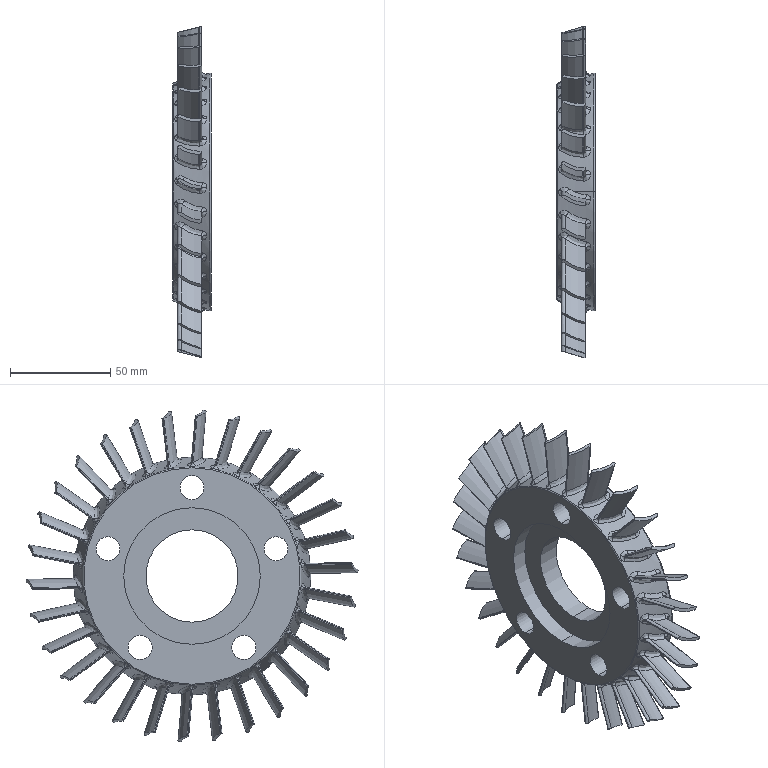Part | STEP file | Previa 01.sldasm-Part-14_Valor predeterminado | 1 solid | 503 faces | box 19 x 165.343 x 165.042 mm | volume 149848 mm3 | cylinder 224 | spline 210 | plane 33 | cone 32 | torus 4 | commonest cylinder face diameters 2.56 x90 0.64 x60 34.26 x30 37.46 x30 12 x10 46 x2